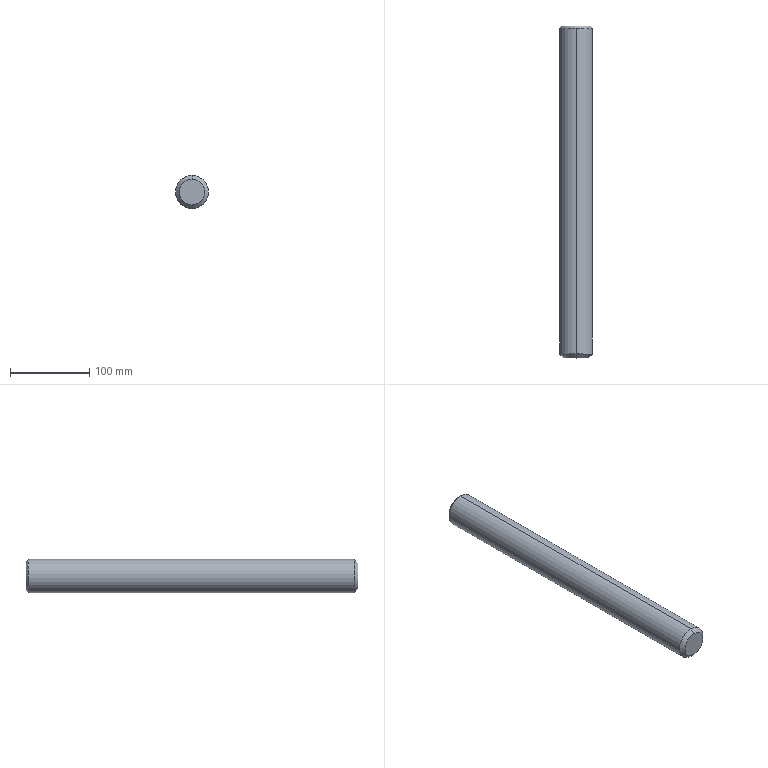Part | SolidWorks | features Chamfer 2, Extrusion 1 | 1 solid | 8 faces | box 42 x 420 x 42 mm | volume 579802 mm3 | cone 4 | cylinder 2 | plane 2 | commonest cylinder face diameters 42 x2
STEP:
#1=CARTESIAN_POINT('',(0.,420.,18.));
#2=VERTEX_POINT('',#1);
#3=CARTESIAN_POINT('',(0.,420.,-18.));
#4=VERTEX_POINT('',#3);
#5=CARTESIAN_POINT('',(0.,420.,0.));
#6=DIRECTION('',(0.,1.,0.));
#7=DIRECTION('',(0.,0.,1.));
#8=AXIS2_PLACEMENT_3D('',#5,#6,#7);
#9=CIRCLE('',#8,18.);
#10=EDGE_CURVE('',#2,#4,#9,.T.);
#11=ORIENTED_EDGE('',*,*,#10,.F.);
#12=CARTESIAN_POINT('',(0.,417.,21.));
#13=VERTEX_POINT('',#12);
#14=CARTESIAN_POINT('',(0.,420.,18.));
#15=DIRECTION('',(0.,-0.7071,0.7071));
#16=VECTOR('',#15,1000.);
#17=LINE('',#14,#16);
#18=EDGE_CURVE('',#2,#13,#17,.T.);
#19=ORIENTED_EDGE('',*,*,#18,.T.);
#20=CARTESIAN_POINT('',(0.,417.,-21.));
#21=VERTEX_POINT('',#20);
#22=CARTESIAN_POINT('',(0.,417.,0.));
#23=DIRECTION('',(0.,-1.,0.));
#24=DIRECTION('',(0.,0.,1.));
#25=AXIS2_PLACEMENT_3D('',#22,#23,#24);
#26=CIRCLE('',#25,21.);
#27=EDGE_CURVE('',#21,#13,#26,.T.);
#28=ORIENTED_EDGE('',*,*,#27,.F.);
#29=CARTESIAN_POINT('',(0.,420.,-18.));
#30=DIRECTION('',(0.,-0.7071,-0.7071));
#31=VECTOR('',#30,1000.);
#32=LINE('',#29,#31);
#33=EDGE_CURVE('',#4,#21,#32,.T.);
#34=ORIENTED_EDGE('',*,*,#33,.F.);
#35=EDGE_LOOP('',(#11,#19,#28,#34));
#36=FACE_OUTER_BOUND('',#35,.T.);
#37=CARTESIAN_POINT('',(0.,420.,0.));
#38=DIRECTION('',(0.,-1.,0.));
#39=DIRECTION('',(0.,0.,-1.));
#40=AXIS2_PLACEMENT_3D('',#37,#38,#39);
#41=CONICAL_SURFACE('',#40,18.,0.7854);
#42=ADVANCED_FACE('',(#36),#41,.T.);
#43=CARTESIAN_POINT('',(0.,0.,-16.));
#44=VERTEX_POINT('',#43);
#45=CARTESIAN_POINT('',(0.,0.,16.));
#46=VERTEX_POINT('',#45);
#47=CARTESIAN_POINT('',(0.,0.,0.));
#48=DIRECTION('',(0.,-1.,0.));
#49=DIRECTION('',(0.,0.,1.));
#50=AXIS2_PLACEMENT_3D('',#47,#48,#49);
#51=CIRCLE('',#50,16.);
#52=EDGE_CURVE('',#44,#46,#51,.T.);
#53=ORIENTED_EDGE('',*,*,#52,.F.);
#54=CARTESIAN_POINT('',(0.,5.,-21.));
#55=VERTEX_POINT('',#54);
#56=CARTESIAN_POINT('',(0.,5.,-21.));
#57=DIRECTION('',(0.,0.7071,-0.7071));
#58=VECTOR('',#57,1000.);
#59=LINE('',#56,#58);
#60=EDGE_CURVE('',#44,#55,#59,.T.);
#61=ORIENTED_EDGE('',*,*,#60,.T.);
#62=CARTESIAN_POINT('',(0.,5.,21.));
#63=VERTEX_POINT('',#62);
#64=CARTESIAN_POINT('',(0.,5.,0.));
#65=DIRECTION('',(0.,1.,0.));
#66=DIRECTION('',(0.,0.,1.));
#67=AXIS2_PLACEMENT_3D('',#64,#65,#66);
#68=CIRCLE('',#67,21.);
#69=EDGE_CURVE('',#63,#55,#68,.T.);
#70=ORIENTED_EDGE('',*,*,#69,.F.);
#71=CARTESIAN_POINT('',(0.,5.,21.));
#72=DIRECTION('',(0.,0.7071,0.7071));
#73=VECTOR('',#72,1000.);
#74=LINE('',#71,#73);
#75=EDGE_CURVE('',#46,#63,#74,.T.);
#76=ORIENTED_EDGE('',*,*,#75,.F.);
#77=EDGE_LOOP('',(#53,#61,#70,#76));
#78=FACE_OUTER_BOUND('',#77,.T.);
#79=CARTESIAN_POINT('',(0.,5.,0.));
#80=DIRECTION('',(0.,1.,0.));
#81=DIRECTION('',(0.,0.,1.));
#82=AXIS2_PLACEMENT_3D('',#79,#80,#81);
#83=CONICAL_SURFACE('',#82,21.,0.7854);
#84=ADVANCED_FACE('',(#78),#83,.T.);
#85=ORIENTED_EDGE('',*,*,#27,.T.);
#86=CARTESIAN_POINT('',(0.,420.,21.));
#87=DIRECTION('',(0.,-1.,0.));
#88=VECTOR('',#87,1000.);
#89=LINE('',#86,#88);
#90=EDGE_CURVE('',#13,#63,#89,.T.);
#91=ORIENTED_EDGE('',*,*,#90,.T.);
#92=ORIENTED_EDGE('',*,*,#69,.T.);
#93=CARTESIAN_POINT('',(0.,420.,-21.));
#94=DIRECTION('',(0.,-1.,0.));
#95=VECTOR('',#94,1000.);
#96=LINE('',#93,#95);
#97=EDGE_CURVE('',#21,#55,#96,.T.);
#98=ORIENTED_EDGE('',*,*,#97,.F.);
#99=EDGE_LOOP('',(#85,#91,#92,#98));
#100=FACE_OUTER_BOUND('',#99,.T.);
#101=CARTESIAN_POINT('',(0.,420.,0.));
#102=DIRECTION('',(0.,-1.,0.));
#103=DIRECTION('',(0.,0.,-1.));
#104=AXIS2_PLACEMENT_3D('',#101,#102,#103);
#105=CYLINDRICAL_SURFACE('',#104,21.);
#106=ADVANCED_FACE('',(#100),#105,.T.);
#107=ORIENTED_EDGE('',*,*,#90,.F.);
#108=CARTESIAN_POINT('',(0.,417.,0.));
#109=DIRECTION('',(0.,-1.,0.));
#110=DIRECTION('',(0.,0.,1.));
#111=AXIS2_PLACEMENT_3D('',#108,#109,#110);
#112=CIRCLE('',#111,21.);
#113=EDGE_CURVE('',#13,#21,#112,.T.);
#114=ORIENTED_EDGE('',*,*,#113,.T.);
#115=ORIENTED_EDGE('',*,*,#97,.T.);
#116=CARTESIAN_POINT('',(0.,5.,0.));
#117=DIRECTION('',(0.,1.,0.));
#118=DIRECTION('',(0.,0.,1.));
#119=AXIS2_PLACEMENT_3D('',#116,#117,#118);
#120=CIRCLE('',#119,21.);
#121=EDGE_CURVE('',#55,#63,#120,.T.);
#122=ORIENTED_EDGE('',*,*,#121,.T.);
#123=EDGE_LOOP('',(#107,#114,#115,#122));
#124=FACE_OUTER_BOUND('',#123,.T.);
#125=CARTESIAN_POINT('',(0.,420.,0.));
#126=DIRECTION('',(0.,-1.,0.));
#127=DIRECTION('',(0.,0.,-1.));
#128=AXIS2_PLACEMENT_3D('',#125,#126,#127);
#129=CYLINDRICAL_SURFACE('',#128,21.);
#130=ADVANCED_FACE('',(#124),#129,.T.);
#131=CARTESIAN_POINT('',(0.,420.,0.));
#132=DIRECTION('',(0.,1.,0.));
#133=DIRECTION('',(0.,0.,1.));
#134=AXIS2_PLACEMENT_3D('',#131,#132,#133);
#135=CIRCLE('',#134,18.);
#136=EDGE_CURVE('',#4,#2,#135,.T.);
#137=ORIENTED_EDGE('',*,*,#136,.T.);
#138=ORIENTED_EDGE('',*,*,#10,.T.);
#139=EDGE_LOOP('',(#137,#138));
#140=FACE_OUTER_BOUND('',#139,.T.);
#141=CARTESIAN_POINT('',(0.,420.,0.));
#142=DIRECTION('',(0.,1.,0.));
#143=DIRECTION('',(0.,0.,1.));
#144=AXIS2_PLACEMENT_3D('',#141,#142,#143);
#145=PLANE('',#144);
#146=ADVANCED_FACE('',(#140),#145,.T.);
#147=CARTESIAN_POINT('',(0.,0.,0.));
#148=DIRECTION('',(0.,-1.,0.));
#149=DIRECTION('',(0.,0.,1.));
#150=AXIS2_PLACEMENT_3D('',#147,#148,#149);
#151=CIRCLE('',#150,16.);
#152=EDGE_CURVE('',#46,#44,#151,.T.);
#153=ORIENTED_EDGE('',*,*,#152,.T.);
#154=ORIENTED_EDGE('',*,*,#52,.T.);
#155=EDGE_LOOP('',(#153,#154));
#156=FACE_OUTER_BOUND('',#155,.T.);
#157=CARTESIAN_POINT('',(0.,0.,0.));
#158=DIRECTION('',(0.,1.,0.));
#159=DIRECTION('',(0.,0.,1.));
#160=AXIS2_PLACEMENT_3D('',#157,#158,#159);
#161=PLANE('',#160);
#162=ADVANCED_FACE('',(#156),#161,.F.);
#163=ORIENTED_EDGE('',*,*,#60,.F.);
#164=ORIENTED_EDGE('',*,*,#152,.F.);
#165=ORIENTED_EDGE('',*,*,#75,.T.);
#166=ORIENTED_EDGE('',*,*,#121,.F.);
#167=EDGE_LOOP('',(#163,#164,#165,#166));
#168=FACE_OUTER_BOUND('',#167,.T.);
#169=CARTESIAN_POINT('',(0.,5.,0.));
#170=DIRECTION('',(0.,1.,0.));
#171=DIRECTION('',(0.,0.,1.));
#172=AXIS2_PLACEMENT_3D('',#169,#170,#171);
#173=CONICAL_SURFACE('',#172,21.,0.7854);
#174=ADVANCED_FACE('',(#168),#173,.T.);
#175=ORIENTED_EDGE('',*,*,#18,.F.);
#176=ORIENTED_EDGE('',*,*,#136,.F.);
#177=ORIENTED_EDGE('',*,*,#33,.T.);
#178=ORIENTED_EDGE('',*,*,#113,.F.);
#179=EDGE_LOOP('',(#175,#176,#177,#178));
#180=FACE_OUTER_BOUND('',#179,.T.);
#181=CARTESIAN_POINT('',(0.,420.,0.));
#182=DIRECTION('',(0.,-1.,0.));
#183=DIRECTION('',(0.,0.,-1.));
#184=AXIS2_PLACEMENT_3D('',#181,#182,#183);
#185=CONICAL_SURFACE('',#184,18.,0.7854);
#186=ADVANCED_FACE('',(#180),#185,.T.);
#187=CLOSED_SHELL('',(#42,#84,#106,#130,#146,#162,#174,#186));
#188=MANIFOLD_SOLID_BREP('',#187);
#189=CARTESIAN_POINT('',(0.,0.,0.));
#190=DIRECTION('',(0.,0.,1.));
#191=DIRECTION('',(1.,0.,0.));
#192=AXIS2_PLACEMENT_3D('',#189,#190,#191);
#193=(LENGTH_UNIT()NAMED_UNIT(*)SI_UNIT(.MILLI.,.METRE.));
#194=UNCERTAINTY_MEASURE_WITH_UNIT(LENGTH_MEASURE(0.00001),#193,'','');
#195=(NAMED_UNIT(*)PLANE_ANGLE_UNIT()SI_UNIT($,.RADIAN.));
#196=(NAMED_UNIT(*)SI_UNIT($,.STERADIAN.)SOLID_ANGLE_UNIT());
#197=(GEOMETRIC_REPRESENTATION_CONTEXT(3)GLOBAL_UNCERTAINTY_ASSIGNED_CONTEXT((#194))GLOBAL_UNIT_ASSIGNED_CONTEXT((#193,#195,#196))REPRESENTATION_CONTEXT('',''));
#198=ADVANCED_BREP_SHAPE_REPRESENTATION('',(#188,#192),#197);